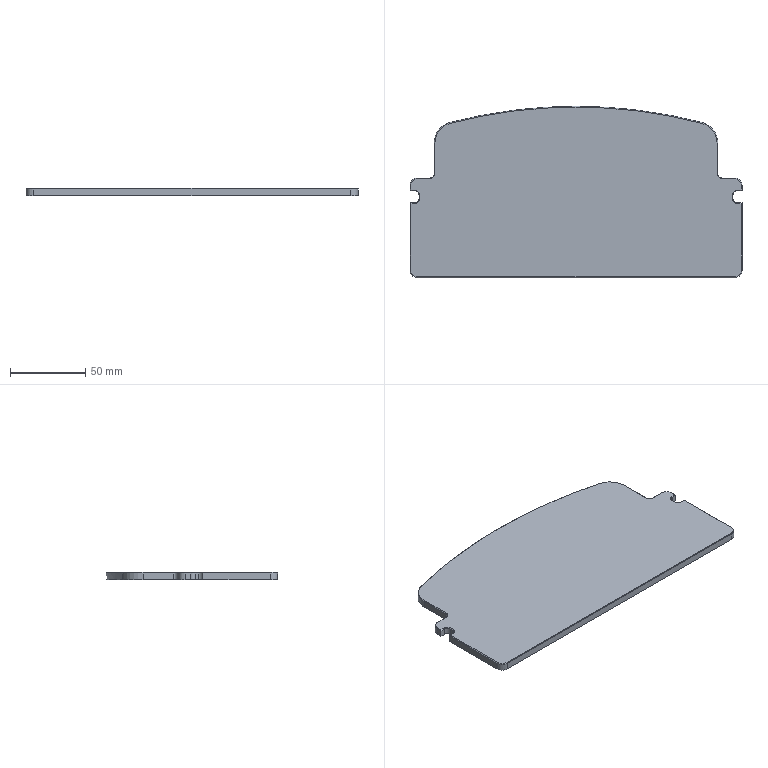Part | SolidWorks | features BaseBody 1 | 1 solid | 59 faces | box 220 x 113.5 x 5 mm | volume 112175 mm3 | plane 32 | cone 14 | cylinder 13 | commonest cylinder face diameters 6 x6 10 x4 28 x2 660 x1